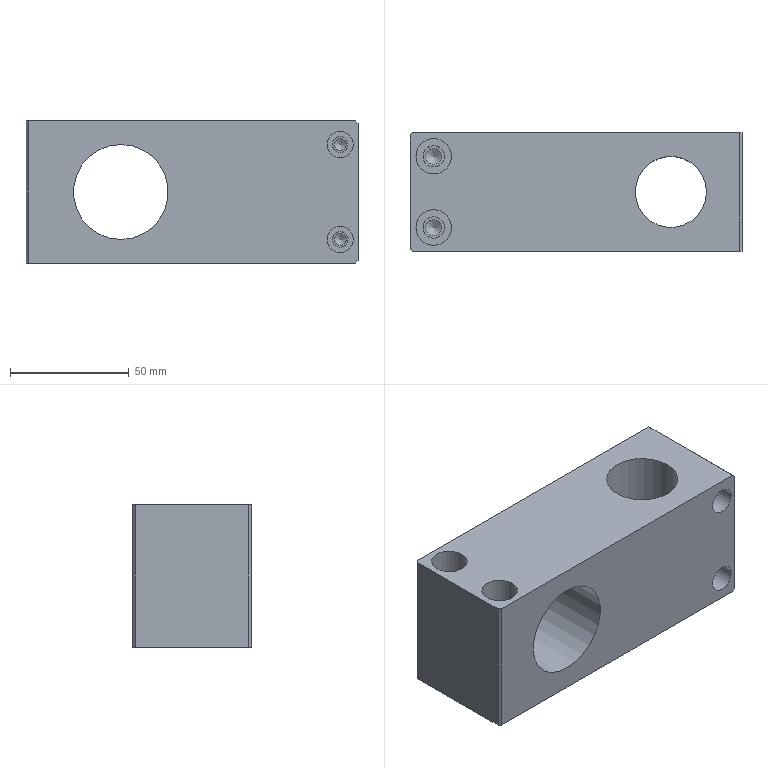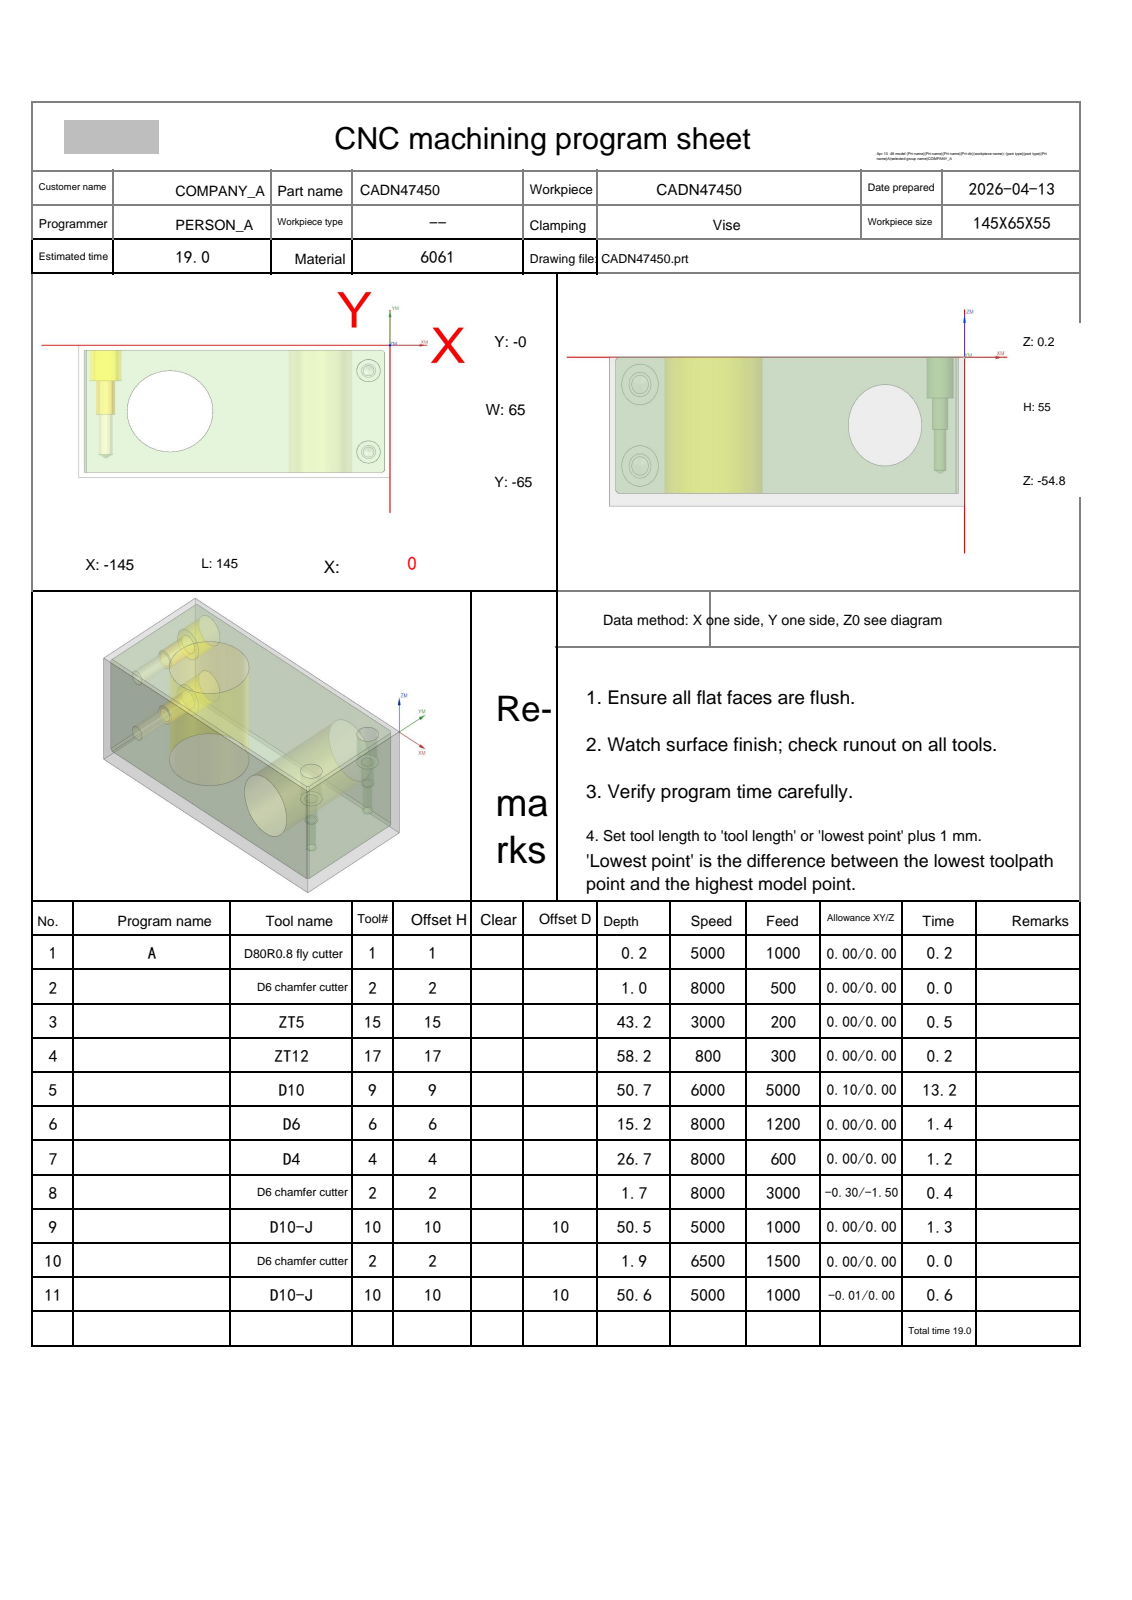NC program | NX | posted by the shop | part box 140 x 50 x 60 mm
Lines 77 to 885 of 4750:
N5 T09 M06
(D10  D=10. R=0. H=09 ce=0.10 di=0.00)
G00 G90 G54 X-73. Y2.6 M03 S6000
G43 H09 Z20.
M08
Z.5
G01 X-3.5 Z.372 F5000.
G02 X.106 Y1.106 Z.365 I0.0 J-5.1
G01 X1.106 Y.106 Z.362
G02 X2.6 Y-3.5 Z.355 I-3.606 J-3.606
G01 Y-61.5 Z.248
G02 X1.106 Y-65.106 Z.24 I-5.1 J0.0
G01 X.106 Y-66.106 Z.238
G02 X-3.5 Y-67.6 Z.23 I-3.606 J3.606
G01 X-142.5 Z-.026
G02 X-147.6 Y-62.5 Z-.04 I0.0 J5.1
G01 Y-2.5 Z-.151
G02 X-142.5 Y2.6 Z-.166 I5.1 J0.0
G01 X-3.5 Z-.422
G02 X.106 Y1.106 Z-.429 I0.0 J-5.1
G01 X1.106 Y.106 Z-.432
G02 X2.6 Y-3.5 Z-.439 I-3.606 J-3.606
G01 Y-61.5 Z-.546
G02 X1.106 Y-65.106 Z-.553 I-5.1 J0.0
G01 X.106 Y-66.106 Z-.556
G02 X-3.5 Y-67.6 Z-.563 I-3.606 J3.606
G01 X-142.5 Z-.819
G02 X-147.6 Y-62.5 Z-.834 I0.0 J5.1
G01 Y-2.5 Z-.945
G02 X-142.5 Y2.6 Z-.959 I5.1 J0.0
G01 X-3.5 Z-1.216
G02 X.106 Y1.106 Z-1.223 I0.0 J-5.1
G01 X1.106 Y.106 Z-1.226
G02 X2.6 Y-3.5 Z-1.233 I-3.606 J-3.606
G01 Y-61.5 Z-1.34
G02 X1.106 Y-65.106 Z-1.347 I-5.1 J0.0
G01 X.106 Y-66.106 Z-1.35
G02 X-3.5 Y-67.6 Z-1.357 I-3.606 J3.606
G01 X-142.5 Z-1.613
G02 X-147.6 Y-62.5 Z-1.628 I0.0 J5.1
G01 Y-2.5 Z-1.738
G02 X-142.5 Y2.6 Z-1.753 I5.1 J0.0
G01 X-3.5 Z-2.009
G02 X.106 Y1.106 Z-2.017 I0.0 J-5.1
G01 X1.106 Y.106 Z-2.019
G02 X2.6 Y-3.5 Z-2.027 I-3.606 J-3.606
G01 Y-61.5 Z-2.133
G02 X1.106 Y-65.106 Z-2.141 I-5.1 J0.0
G01 X.106 Y-66.106 Z-2.143
G02 X-3.5 Y-67.6 Z-2.151 I-3.606 J3.606
G01 X-142.5 Z-2.407
G02 X-147.6 Y-62.5 Z-2.422 I0.0 J5.1
G01 Y-2.5 Z-2.532
G02 X-142.5 Y2.6 Z-2.547 I5.1 J0.0
G01 X-3.5 Z-2.803
G02 X.106 Y1.106 Z-2.81 I0.0 J-5.1
G01 X1.106 Y.106 Z-2.813
G02 X2.6 Y-3.5 Z-2.82 I-3.606 J-3.606
G01 Y-61.5 Z-2.927
G02 X1.106 Y-65.106 Z-2.935 I-5.1 J0.0
G01 X.106 Y-66.106 Z-2.937
G02 X-3.5 Y-67.6 Z-2.945 I-3.606 J3.606
G01 X-142.5 Z-3.201
G02 X-147.6 Y-62.5 Z-3.215 I0.0 J5.1
G01 Y-2.5 Z-3.326
G02 X-142.5 Y2.6 Z-3.341 I5.1 J0.0
G01 X-3.5 Z-3.597
G02 X.106 Y1.106 Z-3.604 I0.0 J-5.1
G01 X1.106 Y.106 Z-3.607
G02 X2.6 Y-3.5 Z-3.614 I-3.606 J-3.606
G01 Y-61.5 Z-3.721
G02 X1.106 Y-65.106 Z-3.728 I-5.1 J0.0
G01 X.106 Y-66.106 Z-3.731
G02 X-3.5 Y-67.6 Z-3.738 I-3.606 J3.606
G01 X-142.5 Z-3.994
G02 X-147.6 Y-62.5 Z-4.009 I0.0 J5.1
G01 Y-2.5 Z-4.12
G02 X-142.5 Y2.6 Z-4.134 I5.1 J0.0
G01 X-3.5 Z-4.391
G02 X.106 Y1.106 Z-4.398 I0.0 J-5.1
G01 X1.106 Y.106 Z-4.401
G02 X2.6 Y-3.5 Z-4.408 I-3.606 J-3.606
G01 Y-61.5 Z-4.515
G02 X1.106 Y-65.106 Z-4.522 I-5.1 J0.0
G01 X.106 Y-66.106 Z-4.525
G02 X-3.5 Y-67.6 Z-4.532 I-3.606 J3.606
G01 X-142.5 Z-4.788
G02 X-147.6 Y-62.5 Z-4.803 I0.0 J5.1
G01 Y-2.5 Z-4.913
G02 X-142.5 Y2.6 Z-4.928 I5.1 J0.0
G01 X-3.5 Z-5.184
G02 X.106 Y1.106 Z-5.192 I0.0 J-5.1
G01 X1.106 Y.106 Z-5.194
G02 X2.6 Y-3.5 Z-5.202 I-3.606 J-3.606
G01 Y-61.5 Z-5.308
G02 X1.106 Y-65.106 Z-5.316 I-5.1 J0.0
G01 X.106 Y-66.106 Z-5.318
G02 X-3.5 Y-67.6 Z-5.326 I-3.606 J3.606
G01 X-142.5 Z-5.582
G02 X-147.6 Y-62.5 Z-5.597 I0.0 J5.1
G01 Y-2.5 Z-5.707
G02 X-142.5 Y2.6 Z-5.722 I5.1 J0.0
G01 X-3.5 Z-5.978
G02 X.106 Y1.106 Z-5.985 I0.0 J-5.1
G01 X1.106 Y.106 Z-5.988
G02 X2.6 Y-3.5 Z-5.995 I-3.606 J-3.606
G01 Y-61.5 Z-6.102
G02 X1.106 Y-65.106 Z-6.11 I-5.1 J0.0
G01 X.106 Y-66.106 Z-6.112
G02 X-3.5 Y-67.6 Z-6.12 I-3.606 J3.606
G01 X-142.5 Z-6.376
G02 X-147.6 Y-62.5 Z-6.39 I0.0 J5.1
G01 Y-2.5 Z-6.501
G02 X-142.5 Y2.6 Z-6.516 I5.1 J0.0
G01 X-3.5 Z-6.772
G02 X.106 Y1.106 Z-6.779 I0.0 J-5.1
G01 X1.106 Y.106 Z-6.782
G02 X2.6 Y-3.5 Z-6.789 I-3.606 J-3.606
G01 Y-61.5 Z-6.896
G02 X1.106 Y-65.106 Z-6.903 I-5.1 J0.0
G01 X.106 Y-66.106 Z-6.906
G02 X-3.5 Y-67.6 Z-6.913 I-3.606 J3.606
G01 X-142.5 Z-7.169
G02 X-147.6 Y-62.5 Z-7.184 I0.0 J5.1
G01 Y-2.5 Z-7.295
G02 X-142.5 Y2.6 Z-7.309 I5.1 J0.0
G01 X-3.5 Z-7.566
G02 X.106 Y1.106 Z-7.573 I0.0 J-5.1
G01 X1.106 Y.106 Z-7.576
G02 X2.6 Y-3.5 Z-7.583 I-3.606 J-3.606
G01 Y-61.5 Z-7.69
G02 X1.106 Y-65.106 Z-7.697 I-5.1 J0.0
G01 X.106 Y-66.106 Z-7.7
G02 X-3.5 Y-67.6 Z-7.707 I-3.606 J3.606
G01 X-142.5 Z-7.963
G02 X-147.6 Y-62.5 Z-7.978 I0.0 J5.1
G01 Y-2.5 Z-8.088
G02 X-142.5 Y2.6 Z-8.103 I5.1 J0.0
G01 X-3.5 Z-8.359
G02 X.106 Y1.106 Z-8.367 I0.0 J-5.1
G01 X1.106 Y.106 Z-8.369
G02 X2.6 Y-3.5 Z-8.377 I-3.606 J-3.606
G01 Y-61.5 Z-8.483
G02 X1.106 Y-65.106 Z-8.491 I-5.1 J0.0
G01 X.106 Y-66.106 Z-8.493
G02 X-3.5 Y-67.6 Z-8.501 I-3.606 J3.606
G01 X-142.5 Z-8.757
G02 X-147.6 Y-62.5 Z-8.772 I0.0 J5.1
G01 Y-2.5 Z-8.882
G02 X-142.5 Y2.6 Z-8.897 I5.1 J0.0
G01 X-3.5 Z-9.153
G02 X.106 Y1.106 Z-9.16 I0.0 J-5.1
G01 X1.106 Y.106 Z-9.163
G02 X2.6 Y-3.5 Z-9.17 I-3.606 J-3.606
G01 Y-61.5 Z-9.277
G02 X1.106 Y-65.106 Z-9.285 I-5.1 J0.0
G01 X.106 Y-66.106 Z-9.287
G02 X-3.5 Y-67.6 Z-9.295 I-3.606 J3.606
G01 X-142.5 Z-9.551
G02 X-147.6 Y-62.5 Z-9.565 I0.0 J5.1
G01 Y-2.5 Z-9.676
G02 X-142.5 Y2.6 Z-9.691 I5.1 J0.0
G01 X-3.5 Z-9.947
G02 X.106 Y1.106 Z-9.954 I0.0 J-5.1
G01 X1.106 Y.106 Z-9.957
G02 X2.6 Y-3.5 Z-9.964 I-3.606 J-3.606
G01 Y-61.5 Z-10.071
G02 X1.106 Y-65.106 Z-10.078 I-5.1 J0.0
G01 X.106 Y-66.106 Z-10.081
G02 X-3.5 Y-67.6 Z-10.088 I-3.606 J3.606
G01 X-142.5 Z-10.344
G02 X-147.6 Y-62.5 Z-10.359 I0.0 J5.1
G01 Y-2.5 Z-10.47
G02 X-142.5 Y2.6 Z-10.484 I5.1 J0.0
G01 X-3.5 Z-10.741
G02 X.106 Y1.106 Z-10.748 I0.0 J-5.1
G01 X1.106 Y.106 Z-10.751
G02 X2.6 Y-3.5 Z-10.758 I-3.606 J-3.606
G01 Y-61.5 Z-10.865
G02 X1.106 Y-65.106 Z-10.872 I-5.1 J0.0
G01 X.106 Y-66.106 Z-10.875
G02 X-3.5 Y-67.6 Z-10.882 I-3.606 J3.606
G01 X-142.5 Z-11.138
G02 X-147.6 Y-62.5 Z-11.153 I0.0 J5.1
G01 Y-2.5 Z-11.263
G02 X-142.5 Y2.6 Z-11.278 I5.1 J0.0
G01 X-3.5 Z-11.534
G02 X.106 Y1.106 Z-11.542 I0.0 J-5.1
G01 X1.106 Y.106 Z-11.544
G02 X2.6 Y-3.5 Z-11.552 I-3.606 J-3.606
G01 Y-61.5 Z-11.658
G02 X1.106 Y-65.106 Z-11.666 I-5.1 J0.0
G01 X.106 Y-66.106 Z-11.668
G02 X-3.5 Y-67.6 Z-11.676 I-3.606 J3.606
G01 X-142.5 Z-11.932
G02 X-147.6 Y-62.5 Z-11.947 I0.0 J5.1
G01 Y-2.5 Z-12.057
G02 X-142.5 Y2.6 Z-12.072 I5.1 J0.0
G01 X-3.5 Z-12.328
G02 X.106 Y1.106 Z-12.335 I0.0 J-5.1
G01 X1.106 Y.106 Z-12.338
G02 X2.6 Y-3.5 Z-12.345 I-3.606 J-3.606
G01 Y-61.5 Z-12.452
G02 X1.106 Y-65.106 Z-12.46 I-5.1 J0.0
G01 X.106 Y-66.106 Z-12.462
G02 X-3.5 Y-67.6 Z-12.47 I-3.606 J3.606
G01 X-142.5 Z-12.726
G02 X-147.6 Y-62.5 Z-12.74 I0.0 J5.1
G01 Y-2.5 Z-12.851
G02 X-142.5 Y2.6 Z-12.866 I5.1 J0.0
G01 X-3.5 Z-13.122
G02 X.106 Y1.106 Z-13.129 I0.0 J-5.1
G01 X1.106 Y.106 Z-13.132
G02 X2.6 Y-3.5 Z-13.139 I-3.606 J-3.606
G01 Y-61.5 Z-13.246
G02 X1.106 Y-65.106 Z-13.253 I-5.1 J0.0
G01 X.106 Y-66.106 Z-13.256
G02 X-3.5 Y-67.6 Z-13.263 I-3.606 J3.606
G01 X-142.5 Z-13.519
G02 X-147.6 Y-62.5 Z-13.534 I0.0 J5.1
G01 Y-2.5 Z-13.645
G02 X-142.5 Y2.6 Z-13.659 I5.1 J0.0
G01 X-3.5 Z-13.916
G02 X.106 Y1.106 Z-13.923 I0.0 J-5.1
G01 X1.106 Y.106 Z-13.926
G02 X2.6 Y-3.5 Z-13.933 I-3.606 J-3.606
G01 Y-61.5 Z-14.04
G02 X1.106 Y-65.106 Z-14.047 I-5.1 J0.0
G01 X.106 Y-66.106 Z-14.05
G02 X-3.5 Y-67.6 Z-14.057 I-3.606 J3.606
G01 X-142.5 Z-14.313
G02 X-147.6 Y-62.5 Z-14.328 I0.0 J5.1
G01 Y-2.5 Z-14.438
G02 X-142.5 Y2.6 Z-14.453 I5.1 J0.0
G01 X-3.5 Z-14.709
G02 X.106 Y1.106 Z-14.717 I0.0 J-5.1
G01 X1.106 Y.106 Z-14.719
G02 X2.6 Y-3.5 Z-14.727 I-3.606 J-3.606
G01 Y-61.5 Z-14.833
G02 X1.106 Y-65.106 Z-14.841 I-5.1 J0.0
G01 X.106 Y-66.106 Z-14.843
G02 X-3.5 Y-67.6 Z-14.851 I-3.606 J3.606
G01 X-142.5 Z-15.107
G02 X-147.6 Y-62.5 Z-15.122 I0.0 J5.1
G01 Y-2.5 Z-15.232
G02 X-142.5 Y2.6 Z-15.247 I5.1 J0.0
G01 X-3.5 Z-15.503
G02 X.106 Y1.106 Z-15.51 I0.0 J-5.1
G01 X1.106 Y.106 Z-15.513
G02 X2.6 Y-3.5 Z-15.52 I-3.606 J-3.606
G01 Y-61.5 Z-15.627
G02 X1.106 Y-65.106 Z-15.635 I-5.1 J0.0
G01 X.106 Y-66.106 Z-15.637
G02 X-3.5 Y-67.6 Z-15.645 I-3.606 J3.606
G01 X-142.5 Z-15.901
G02 X-147.6 Y-62.5 Z-15.915 I0.0 J5.1
G01 Y-2.5 Z-16.026
G02 X-142.5 Y2.6 Z-16.041 I5.1 J0.0
G01 X-3.5 Z-16.297
G02 X.106 Y1.106 Z-16.304 I0.0 J-5.1
G01 X1.106 Y.106 Z-16.307
G02 X2.6 Y-3.5 Z-16.314 I-3.606 J-3.606
G01 Y-61.5 Z-16.421
G02 X1.106 Y-65.106 Z-16.428 I-5.1 J0.0
G01 X.106 Y-66.106 Z-16.431
G02 X-3.5 Y-67.6 Z-16.438 I-3.606 J3.606
G01 X-142.5 Z-16.694
G02 X-147.6 Y-62.5 Z-16.709 I0.0 J5.1
G01 Y-2.5 Z-16.82
G02 X-142.5 Y2.6 Z-16.834 I5.1 J0.0
G01 X-3.5 Z-17.091
G02 X.106 Y1.106 Z-17.098 I0.0 J-5.1
G01 X1.106 Y.106 Z-17.101
G02 X2.6 Y-3.5 Z-17.108 I-3.606 J-3.606
G01 Y-61.5 Z-17.215
G02 X1.106 Y-65.106 Z-17.222 I-5.1 J0.0
G01 X.106 Y-66.106 Z-17.225
G02 X-3.5 Y-67.6 Z-17.232 I-3.606 J3.606
G01 X-142.5 Z-17.488
G02 X-147.6 Y-62.5 Z-17.503 I0.0 J5.1
G01 Y-2.5 Z-17.613
G02 X-142.5 Y2.6 Z-17.628 I5.1 J0.0
G01 X-3.5 Z-17.884
G02 X.106 Y1.106 Z-17.892 I0.0 J-5.1
G01 X1.106 Y.106 Z-17.894
G02 X2.6 Y-3.5 Z-17.902 I-3.606 J-3.606
G01 Y-61.5 Z-18.008
G02 X1.106 Y-65.106 Z-18.016 I-5.1 J0.0
G01 X.106 Y-66.106 Z-18.018
G02 X-3.5 Y-67.6 Z-18.026 I-3.606 J3.606
G01 X-142.5 Z-18.282
G02 X-147.6 Y-62.5 Z-18.297 I0.0 J5.1
G01 Y-2.5 Z-18.407
G02 X-142.5 Y2.6 Z-18.422 I5.1 J0.0
G01 X-3.5 Z-18.678
G02 X.106 Y1.106 Z-18.685 I0.0 J-5.1
G01 X1.106 Y.106 Z-18.688
G02 X2.6 Y-3.5 Z-18.695 I-3.606 J-3.606
G01 Y-61.5 Z-18.802
G02 X1.106 Y-65.106 Z-18.81 I-5.1 J0.0
G01 X.106 Y-66.106 Z-18.812
G02 X-3.5 Y-67.6 Z-18.82 I-3.606 J3.606
G01 X-142.5 Z-19.076
G02 X-147.6 Y-62.5 Z-19.09 I0.0 J5.1
G01 Y-2.5 Z-19.201
G02 X-142.5 Y2.6 Z-19.216 I5.1 J0.0
G01 X-3.5 Z-19.472
G02 X.106 Y1.106 Z-19.479 I0.0 J-5.1
G01 X1.106 Y.106 Z-19.482
G02 X2.6 Y-3.5 Z-19.489 I-3.606 J-3.606
G01 Y-61.5 Z-19.596
G02 X1.106 Y-65.106 Z-19.603 I-5.1 J0.0
G01 X.106 Y-66.106 Z-19.606
G02 X-3.5 Y-67.6 Z-19.613 I-3.606 J3.606
G01 X-142.5 Z-19.869
G02 X-147.6 Y-62.5 Z-19.884 I0.0 J5.1
G01 Y-2.5 Z-19.995
G02 X-142.5 Y2.6 Z-20.009 I5.1 J0.0
G01 X-3.5 Z-20.266
G02 X.106 Y1.106 Z-20.273 I0.0 J-5.1
G01 X1.106 Y.106 Z-20.276
G02 X2.6 Y-3.5 Z-20.283 I-3.606 J-3.606
G01 Y-61.5 Z-20.39
G02 X1.106 Y-65.106 Z-20.397 I-5.1 J0.0
G01 X.106 Y-66.106 Z-20.4
G02 X-3.5 Y-67.6 Z-20.407 I-3.606 J3.606
G01 X-142.5 Z-20.663
G02 X-147.6 Y-62.5 Z-20.678 I0.0 J5.1
G01 Y-2.5 Z-20.788
G02 X-142.5 Y2.6 Z-20.803 I5.1 J0.0
G01 X-3.5 Z-21.059
G02 X.106 Y1.106 Z-21.067 I0.0 J-5.1
G01 X1.106 Y.106 Z-21.069
G02 X2.6 Y-3.5 Z-21.077 I-3.606 J-3.606
G01 Y-61.5 Z-21.183
G02 X1.106 Y-65.106 Z-21.191 I-5.1 J0.0
G01 X.106 Y-66.106 Z-21.193
G02 X-3.5 Y-67.6 Z-21.201 I-3.606 J3.606
G01 X-142.5 Z-21.457
G02 X-147.6 Y-62.5 Z-21.472 I0.0 J5.1
G01 Y-2.5 Z-21.582
G02 X-142.5 Y2.6 Z-21.597 I5.1 J0.0
G01 X-3.5 Z-21.853
G02 X.106 Y1.106 Z-21.86 I0.0 J-5.1
G01 X1.106 Y.106 Z-21.863
G02 X2.6 Y-3.5 Z-21.87 I-3.606 J-3.606
G01 Y-61.5 Z-21.977
G02 X1.106 Y-65.106 Z-21.985 I-5.1 J0.0
G01 X.106 Y-66.106 Z-21.987
G02 X-3.5 Y-67.6 Z-21.995 I-3.606 J3.606
G01 X-142.5 Z-22.251
G02 X-147.6 Y-62.5 Z-22.265 I0.0 J5.1
G01 Y-2.5 Z-22.376
G02 X-142.5 Y2.6 Z-22.391 I5.1 J0.0
G01 X-3.5 Z-22.647
G02 X.106 Y1.106 Z-22.654 I0.0 J-5.1
G01 X1.106 Y.106 Z-22.657
G02 X2.6 Y-3.5 Z-22.664 I-3.606 J-3.606
G01 Y-61.5 Z-22.771
G02 X1.106 Y-65.106 Z-22.778 I-5.1 J0.0
G01 X.106 Y-66.106 Z-22.781
G02 X-3.5 Y-67.6 Z-22.788 I-3.606 J3.606
G01 X-142.5 Z-23.044
G02 X-147.6 Y-62.5 Z-23.059 I0.0 J5.1
G01 Y-2.5 Z-23.17
G02 X-142.5 Y2.6 Z-23.184 I5.1 J0.0
G01 X-3.5 Z-23.441
G02 X.106 Y1.106 Z-23.448 I0.0 J-5.1
G01 X1.106 Y.106 Z-23.451
G02 X2.6 Y-3.5 Z-23.458 I-3.606 J-3.606
G01 Y-61.5 Z-23.565
G02 X1.106 Y-65.106 Z-23.572 I-5.1 J0.0
G01 X.106 Y-66.106 Z-23.575
G02 X-3.5 Y-67.6 Z-23.582 I-3.606 J3.606
G01 X-142.5 Z-23.838
G02 X-147.6 Y-62.5 Z-23.853 I0.0 J5.1
G01 Y-2.5 Z-23.963
G02 X-142.5 Y2.6 Z-23.978 I5.1 J0.0
G01 X-3.5 Z-24.234
G02 X.106 Y1.106 Z-24.242 I0.0 J-5.1
G01 X1.106 Y.106 Z-24.244
G02 X2.6 Y-3.5 Z-24.252 I-3.606 J-3.606
G01 Y-61.5 Z-24.358
G02 X1.106 Y-65.106 Z-24.366 I-5.1 J0.0
G01 X.106 Y-66.106 Z-24.368
G02 X-3.5 Y-67.6 Z-24.376 I-3.606 J3.606
G01 X-142.5 Z-24.632
G02 X-147.6 Y-62.5 Z-24.647 I0.0 J5.1
G01 Y-2.5 Z-24.757
G02 X-142.5 Y2.6 Z-24.772 I5.1 J0.0
G01 X-3.5 Z-25.028
G02 X.106 Y1.106 Z-25.035 I0.0 J-5.1
G01 X1.106 Y.106 Z-25.038
G02 X2.6 Y-3.5 Z-25.045 I-3.606 J-3.606
G01 Y-61.5 Z-25.152
G02 X1.106 Y-65.106 Z-25.16 I-5.1 J0.0
G01 X.106 Y-66.106 Z-25.162
G02 X-3.5 Y-67.6 Z-25.17 I-3.606 J3.606
G01 X-142.5 Z-25.426
G02 X-147.6 Y-62.5 Z-25.44 I0.0 J5.1
G01 Y-2.5 Z-25.551
G02 X-142.5 Y2.6 Z-25.566 I5.1 J0.0
G01 X-3.5 Z-25.822
G02 X.106 Y1.106 Z-25.829 I0.0 J-5.1
G01 X1.106 Y.106 Z-25.832
G02 X2.6 Y-3.5 Z-25.839 I-3.606 J-3.606
G01 Y-61.5 Z-25.946
G02 X1.106 Y-65.106 Z-25.953 I-5.1 J0.0
G01 X.106 Y-66.106 Z-25.956
G02 X-3.5 Y-67.6 Z-25.963 I-3.606 J3.606
G01 X-142.5 Z-26.219
G02 X-147.6 Y-62.5 Z-26.234 I0.0 J5.1
G01 Y-2.5 Z-26.345
G02 X-142.5 Y2.6 Z-26.359 I5.1 J0.0
G01 X-3.5 Z-26.616
G02 X.106 Y1.106 Z-26.623 I0.0 J-5.1
G01 X1.106 Y.106 Z-26.626
G02 X2.6 Y-3.5 Z-26.633 I-3.606 J-3.606
G01 Y-61.5 Z-26.74
G02 X1.106 Y-65.106 Z-26.747 I-5.1 J0.0
G01 X.106 Y-66.106 Z-26.75
G02 X-3.5 Y-67.6 Z-26.757 I-3.606 J3.606
G01 X-142.5 Z-27.013
G02 X-147.6 Y-62.5 Z-27.028 I0.0 J5.1
G01 Y-2.5 Z-27.138
G02 X-142.5 Y2.6 Z-27.153 I5.1 J0.0
G01 X-3.5 Z-27.409
G02 X.106 Y1.106 Z-27.417 I0.0 J-5.1
G01 X1.106 Y.106 Z-27.419
G02 X2.6 Y-3.5 Z-27.427 I-3.606 J-3.606
G01 Y-61.5 Z-27.533
G02 X1.106 Y-65.106 Z-27.541 I-5.1 J0.0
G01 X.106 Y-66.106 Z-27.543
G02 X-3.5 Y-67.6 Z-27.551 I-3.606 J3.606
G01 X-142.5 Z-27.807
G02 X-147.6 Y-62.5 Z-27.822 I0.0 J5.1
G01 Y-2.5 Z-27.932
G02 X-142.5 Y2.6 Z-27.947 I5.1 J0.0
G01 X-3.5 Z-28.203
G02 X.106 Y1.106 Z-28.21 I0.0 J-5.1
G01 X1.106 Y.106 Z-28.213
G02 X2.6 Y-3.5 Z-28.22 I-3.606 J-3.606
G01 Y-61.5 Z-28.327
G02 X1.106 Y-65.106 Z-28.335 I-5.1 J0.0
G01 X.106 Y-66.106 Z-28.337
G02 X-3.5 Y-67.6 Z-28.345 I-3.606 J3.606
G01 X-142.5 Z-28.601
G02 X-147.6 Y-62.5 Z-28.615 I0.0 J5.1
G01 Y-2.5 Z-28.726
G02 X-142.5 Y2.6 Z-28.741 I5.1 J0.0
G01 X-3.5 Z-28.997
G02 X.106 Y1.106 Z-29.004 I0.0 J-5.1
G01 X1.106 Y.106 Z-29.007
G02 X2.6 Y-3.5 Z-29.014 I-3.606 J-3.606
G01 Y-61.5 Z-29.121
G02 X1.106 Y-65.106 Z-29.128 I-5.1 J0.0
G01 X.106 Y-66.106 Z-29.131
G02 X-3.5 Y-67.6 Z-29.138 I-3.606 J3.606
G01 X-142.5 Z-29.394
G02 X-147.6 Y-62.5 Z-29.409 I0.0 J5.1
G01 Y-2.5 Z-29.52
G02 X-142.5 Y2.6 Z-29.534 I5.1 J0.0
G01 X-3.5 Z-29.791
G02 X.106 Y1.106 Z-29.798 I0.0 J-5.1
G01 X1.106 Y.106 Z-29.801
G02 X2.6 Y-3.5 Z-29.808 I-3.606 J-3.606
G01 Y-61.5 Z-29.915
G02 X1.106 Y-65.106 Z-29.922 I-5.1 J0.0
G01 X.106 Y-66.106 Z-29.925
G02 X-3.5 Y-67.6 Z-29.932 I-3.606 J3.606
G01 X-142.5 Z-30.188
G02 X-147.6 Y-62.5 Z-30.203 I0.0 J5.1
G01 Y-2.5 Z-30.313
G02 X-142.5 Y2.6 Z-30.328 I5.1 J0.0
G01 X-3.5 Z-30.584
G02 X.106 Y1.106 Z-30.592 I0.0 J-5.1
G01 X1.106 Y.106 Z-30.594
G02 X2.6 Y-3.5 Z-30.602 I-3.606 J-3.606
G01 Y-61.5 Z-30.708
G02 X1.106 Y-65.106 Z-30.716 I-5.1 J0.0
G01 X.106 Y-66.106 Z-30.718
G02 X-3.5 Y-67.6 Z-30.726 I-3.606 J3.606
G01 X-142.5 Z-30.982
G02 X-147.6 Y-62.5 Z-30.997 I0.0 J5.1
G01 Y-2.5 Z-31.107
G02 X-142.5 Y2.6 Z-31.122 I5.1 J0.0
G01 X-3.5 Z-31.378
G02 X.106 Y1.106 Z-31.385 I0.0 J-5.1
G01 X1.106 Y.106 Z-31.388
G02 X2.6 Y-3.5 Z-31.395 I-3.606 J-3.606
G01 Y-61.5 Z-31.502
G02 X1.106 Y-65.106 Z-31.51 I-5.1 J0.0
G01 X.106 Y-66.106 Z-31.512
G02 X-3.5 Y-67.6 Z-31.52 I-3.606 J3.606
G01 X-142.5 Z-31.776
G02 X-147.6 Y-62.5 Z-31.79 I0.0 J5.1
G01 Y-2.5 Z-31.901
G02 X-142.5 Y2.6 Z-31.916 I5.1 J0.0
G01 X-3.5 Z-32.172
G02 X.106 Y1.106 Z-32.179 I0.0 J-5.1
G01 X1.106 Y.106 Z-32.182
G02 X2.6 Y-3.5 Z-32.189 I-3.606 J-3.606
G01 Y-61.5 Z-32.296
G02 X1.106 Y-65.106 Z-32.303 I-5.1 J0.0
G01 X.106 Y-66.106 Z-32.306
G02 X-3.5 Y-67.6 Z-32.313 I-3.606 J3.606
G01 X-142.5 Z-32.569
G02 X-147.6 Y-62.5 Z-32.584 I0.0 J5.1
G01 Y-2.5 Z-32.695
G02 X-142.5 Y2.6 Z-32.709 I5.1 J0.0
G01 X-3.5 Z-32.966
G02 X.106 Y1.106 Z-32.973 I0.0 J-5.1
G01 X1.106 Y.106 Z-32.976
G02 X2.6 Y-3.5 Z-32.983 I-3.606 J-3.606
G01 Y-61.5 Z-33.09
G02 X1.106 Y-65.106 Z-33.097 I-5.1 J0.0
G01 X.106 Y-66.106 Z-33.1
G02 X-3.5 Y-67.6 Z-33.107 I-3.606 J3.606
G01 X-142.5 Z-33.363
G02 X-147.6 Y-62.5 Z-33.378 I0.0 J5.1
G01 Y-2.5 Z-33.488
G02 X-142.5 Y2.6 Z-33.503 I5.1 J0.0
G01 X-3.5 Z-33.759
G02 X.106 Y1.106 Z-33.767 I0.0 J-5.1
G01 X1.106 Y.106 Z-33.769
G02 X2.6 Y-3.5 Z-33.777 I-3.606 J-3.606
G01 Y-61.5 Z-33.883
G02 X1.106 Y-65.106 Z-33.891 I-5.1 J0.0
G01 X.106 Y-66.106 Z-33.893
G02 X-3.5 Y-67.6 Z-33.901 I-3.606 J3.606
G01 X-142.5 Z-34.157
G02 X-147.6 Y-62.5 Z-34.172 I0.0 J5.1
G01 Y-2.5 Z-34.282
G02 X-142.5 Y2.6 Z-34.297 I5.1 J0.0
G01 X-3.5 Z-34.553
G02 X.106 Y1.106 Z-34.56 I0.0 J-5.1
G01 X1.106 Y.106 Z-34.563
G02 X2.6 Y-3.5 Z-34.57 I-3.606 J-3.606
G01 Y-61.5 Z-34.677
G02 X1.106 Y-65.106 Z-34.685 I-5.1 J0.0
G01 X.106 Y-66.106 Z-34.687
G02 X-3.5 Y-67.6 Z-34.695 I-3.606 J3.606
G01 X-142.5 Z-34.951
G02 X-147.6 Y-62.5 Z-34.965 I0.0 J5.1
G01 Y-2.5 Z-35.076
G02 X-142.5 Y2.6 Z-35.091 I5.1 J0.0
G01 X-3.5 Z-35.347
G02 X.106 Y1.106 Z-35.354 I0.0 J-5.1
G01 X1.106 Y.106 Z-35.357
G02 X2.6 Y-3.5 Z-35.364 I-3.606 J-3.606
G01 Y-61.5 Z-35.471
G02 X1.106 Y-65.106 Z-35.478 I-5.1 J0.0
G01 X.106 Y-66.106 Z-35.481
G02 X-3.5 Y-67.6 Z-35.488 I-3.606 J3.606
G01 X-142.5 Z-35.744
G02 X-147.6 Y-62.5 Z-35.759 I0.0 J5.1
G01 Y-2.5 Z-35.87
G02 X-142.5 Y2.6 Z-35.884 I5.1 J0.0
G01 X-3.5 Z-36.141
G02 X.106 Y1.106 Z-36.148 I0.0 J-5.1
G01 X1.106 Y.106 Z-36.151
G02 X2.6 Y-3.5 Z-36.158 I-3.606 J-3.606
G01 Y-61.5 Z-36.265
G02 X1.106 Y-65.106 Z-36.272 I-5.1 J0.0
G01 X.106 Y-66.106 Z-36.275
G02 X-3.5 Y-67.6 Z-36.282 I-3.606 J3.606
G01 X-142.5 Z-36.538
G02 X-147.6 Y-62.5 Z-36.553 I0.0 J5.1
G01 Y-2.5 Z-36.663
G02 X-142.5 Y2.6 Z-36.678 I5.1 J0.0
G01 X-3.5 Z-36.934
G02 X.106 Y1.106 Z-36.942 I0.0 J-5.1
G01 X1.106 Y.106 Z-36.944
G02 X2.6 Y-3.5 Z-36.952 I-3.606 J-3.606
G01 Y-61.5 Z-37.058
G02 X1.106 Y-65.106 Z-37.066 I-5.1 J0.0
G01 X.106 Y-66.106 Z-37.068
G02 X-3.5 Y-67.6 Z-37.076 I-3.606 J3.606
G01 X-142.5 Z-37.332
G02 X-147.6 Y-62.5 Z-37.347 I0.0 J5.1
G01 Y-2.5 Z-37.457
G02 X-142.5 Y2.6 Z-37.472 I5.1 J0.0
G01 X-3.5 Z-37.728
G02 X.106 Y1.106 Z-37.735 I0.0 J-5.1
G01 X1.106 Y.106 Z-37.738
G02 X2.6 Y-3.5 Z-37.745 I-3.606 J-3.606
G01 Y-61.5 Z-37.852
G02 X1.106 Y-65.106 Z-37.86 I-5.1 J0.0
G01 X.106 Y-66.106 Z-37.862
G02 X-3.5 Y-67.6 Z-37.87 I-3.606 J3.606
G01 X-142.5 Z-38.126
G02 X-147.6 Y-62.5 Z-38.14 I0.0 J5.1
G01 Y-2.5 Z-38.251
G02 X-142.5 Y2.6 Z-38.266 I5.1 J0.0
G01 X-3.5 Z-38.522
G02 X.106 Y1.106 Z-38.529 I0.0 J-5.1
G01 X1.106 Y.106 Z-38.532
G02 X2.6 Y-3.5 Z-38.539 I-3.606 J-3.606
G01 Y-61.5 Z-38.646
G02 X1.106 Y-65.106 Z-38.653 I-5.1 J0.0
G01 X.106 Y-66.106 Z-38.656
G02 X-3.5 Y-67.6 Z-38.663 I-3.606 J3.606
G01 X-142.5 Z-38.919
G02 X-147.6 Y-62.5 Z-38.934 I0.0 J5.1
G01 Y-2.5 Z-39.045
G02 X-142.5 Y2.6 Z-39.059 I5.1 J0.0
G01 X-3.5 Z-39.316
G02 X.106 Y1.106 Z-39.323 I0.0 J-5.1
G01 X1.106 Y.106 Z-39.326
G02 X2.6 Y-3.5 Z-39.333 I-3.606 J-3.606
G01 Y-61.5 Z-39.44
G02 X1.106 Y-65.106 Z-39.447 I-5.1 J0.0
G01 X.106 Y-66.106 Z-39.45
G02 X-3.5 Y-67.6 Z-39.457 I-3.606 J3.606
G01 X-142.5 Z-39.713
G02 X-147.6 Y-62.5 Z-39.728 I0.0 J5.1
G01 Y-2.5 Z-39.838
G02 X-142.5 Y2.6 Z-39.853 I5.1 J0.0
G01 X-3.5 Z-40.109
G02 X.106 Y1.106 Z-40.117 I0.0 J-5.1
G01 X1.106 Y.106 Z-40.119
G02 X2.6 Y-3.5 Z-40.127 I-3.606 J-3.606
G01 Y-61.5 Z-40.233
G02 X1.106 Y-65.106 Z-40.241 I-5.1 J0.0
G01 X.106 Y-66.106 Z-40.243
G02 X-3.5 Y-67.6 Z-40.251 I-3.606 J3.606
G01 X-142.5 Z-40.507
G02 X-147.6 Y-62.5 Z-40.522 I0.0 J5.1
G01 Y-2.5 Z-40.632
G02 X-142.5 Y2.6 Z-40.647 I5.1 J0.0
G01 X-3.5 Z-40.903
G02 X.106 Y1.106 Z-40.91 I0.0 J-5.1
G01 X1.106 Y.106 Z-40.913
G02 X2.6 Y-3.5 Z-40.92 I-3.606 J-3.606
G01 Y-61.5 Z-41.027
G02 X1.106 Y-65.106 Z-41.035 I-5.1 J0.0
G01 X.106 Y-66.106 Z-41.037
G02 X-3.5 Y-67.6 Z-41.045 I-3.606 J3.606
G01 X-142.5 Z-41.301
G02 X-147.6 Y-62.5 Z-41.315 I0.0 J5.1
G01 Y-2.5 Z-41.426
G02 X-142.5 Y2.6 Z-41.441 I5.1 J0.0
G01 X-3.5 Z-41.697
G02 X.106 Y1.106 Z-41.704 I0.0 J-5.1
G01 X1.106 Y.106 Z-41.707
G02 X2.6 Y-3.5 Z-41.714 I-3.606 J-3.606
G01 Y-61.5 Z-41.821
G02 X1.106 Y-65.106 Z-41.828 I-5.1 J0.0
G01 X.106 Y-66.106 Z-41.831
G02 X-3.5 Y-67.6 Z-41.838 I-3.606 J3.606
G01 X-142.5 Z-42.094
G02 X-147.6 Y-62.5 Z-42.109 I0.0 J5.1
G01 Y-2.5 Z-42.22
G02 X-142.5 Y2.6 Z-42.234 I5.1 J0.0
G01 X-3.5 Z-42.491
G02 X.106 Y1.106 Z-42.498 I0.0 J-5.1
G01 X1.106 Y.106 Z-42.501
G02 X2.6 Y-3.5 Z-42.508 I-3.606 J-3.606
G01 Y-61.5 Z-42.615
G02 X1.106 Y-65.106 Z-42.622 I-5.1 J0.0
G01 X.106 Y-66.106 Z-42.625
G02 X-3.5 Y-67.6 Z-42.632 I-3.606 J3.606
G01 X-142.5 Z-42.888
G02 X-147.6 Y-62.5 Z-42.903 I0.0 J5.1
G01 Y-2.5 Z-43.013
G02 X-142.5 Y2.6 Z-43.028 I5.1 J0.0
G01 X-3.5 Z-43.284
G02 X.106 Y1.106 Z-43.292 I0.0 J-5.1
G01 X1.106 Y.106 Z-43.294
G02 X2.6 Y-3.5 Z-43.302 I-3.606 J-3.606
G01 Y-61.5 Z-43.408
G02 X1.106 Y-65.106 Z-43.416 I-5.1 J0.0
G01 X.106 Y-66.106 Z-43.418
G02 X-3.5 Y-67.6 Z-43.426 I-3.606 J3.606
G01 X-142.5 Z-43.682
G02 X-147.6 Y-62.5 Z-43.697 I0.0 J5.1
G01 Y-2.5 Z-43.807
G02 X-142.5 Y2.6 Z-43.822 I5.1 J0.0
G01 X-3.5 Z-44.078
G02 X.106 Y1.106 Z-44.085 I0.0 J-5.1
G01 X1.106 Y.106 Z-44.088
G02 X2.6 Y-3.5 Z-44.095 I-3.606 J-3.606
G01 Y-61.5 Z-44.202
G02 X1.106 Y-65.106 Z-44.21 I-5.1 J0.0
G01 X.106 Y-66.106 Z-44.212
G02 X-3.5 Y-67.6 Z-44.22 I-3.606 J3.606
G01 X-142.5 Z-44.476
G02 X-147.6 Y-62.5 Z-44.49 I0.0 J5.1
G01 Y-2.5 Z-44.601
G02 X-142.5 Y2.6 Z-44.616 I5.1 J0.0
G01 X-3.5 Z-44.872
G02 X.106 Y1.106 Z-44.879 I0.0 J-5.1
G01 X1.106 Y.106 Z-44.882
G02 X2.6 Y-3.5 Z-44.889 I-3.606 J-3.606
G01 Y-61.5 Z-44.996
G02 X1.106 Y-65.106 Z-45.003 I-5.1 J0.0
G01 X.106 Y-66.106 Z-45.006
G02 X-3.5 Y-67.6 Z-45.013 I-3.606 J3.606
G01 X-142.5 Z-45.269
G02 X-147.6 Y-62.5 Z-45.284 I0.0 J5.1
G01 Y-2.5 Z-45.395
G02 X-142.5 Y2.6 Z-45.409 I5.1 J0.0
G01 X-3.5 Z-45.666
G02 X.106 Y1.106 Z-45.673 I0.0 J-5.1
G01 X1.106 Y.106 Z-45.676
G02 X2.6 Y-3.5 Z-45.683 I-3.606 J-3.606
G01 Y-61.5 Z-45.79
G02 X1.106 Y-65.106 Z-45.797 I-5.1 J0.0
G01 X.106 Y-66.106 Z-45.8
G02 X-3.5 Y-67.6 Z-45.807 I-3.606 J3.606
G01 X-142.5 Z-46.063
G02 X-147.6 Y-62.5 Z-46.078 I0.0 J5.1
G01 Y-2.5 Z-46.188
G02 X-142.5 Y2.6 Z-46.203 I5.1 J0.0
G01 X-3.5 Z-46.459
G02 X.106 Y1.106 Z-46.467 I0.0 J-5.1
G01 X1.106 Y.106 Z-46.469
G02 X2.6 Y-3.5 Z-46.477 I-3.606 J-3.606
G01 Y-61.5 Z-46.583
G02 X1.106 Y-65.106 Z-46.591 I-5.1 J0.0
G01 X.106 Y-66.106 Z-46.593
G02 X-3.5 Y-67.6 Z-46.601 I-3.606 J3.606
G01 X-142.5 Z-46.857
G02 X-147.6 Y-62.5 Z-46.872 I0.0 J5.1
G01 Y-2.5 Z-46.982
G02 X-142.5 Y2.6 Z-46.997 I5.1 J0.0
G01 X-3.5 Z-47.253
G02 X.106 Y1.106 Z-47.26 I0.0 J-5.1
G01 X1.106 Y.106 Z-47.263
G02 X2.6 Y-3.5 Z-47.27 I-3.606 J-3.606
G01 Y-61.5 Z-47.377
G02 X1.106 Y-65.106 Z-47.385 I-5.1 J0.0
G01 X.106 Y-66.106 Z-47.387
G02 X-3.5 Y-67.6 Z-47.395 I-3.606 J3.606
G01 X-142.5 Z-47.651
G02 X-147.6 Y-62.5 Z-47.665 I0.0 J5.1
G01 Y-2.5 Z-47.776
G02 X-142.5 Y2.6 Z-47.791 I5.1 J0.0
G01 X-3.5 Z-48.047
G02 X.106 Y1.106 Z-48.054 I0.0 J-5.1
G01 X1.106 Y.106 Z-48.057
G02 X2.6 Y-3.5 Z-48.064 I-3.606 J-3.606
G01 Y-61.5 Z-48.171
G02 X1.106 Y-65.106 Z-48.178 I-5.1 J0.0
G01 X.106 Y-66.106 Z-48.181
G02 X-3.5 Y-67.6 Z-48.188 I-3.606 J3.606
G01 X-142.5 Z-48.444
G02 X-147.6 Y-62.5 Z-48.459 I0.0 J5.1
G01 Y-2.5 Z-48.57
G02 X-142.5 Y2.6 Z-48.584 I5.1 J0.0
G01 X-3.5 Z-48.841
G02 X.106 Y1.106 Z-48.848 I0.0 J-5.1
G01 X1.106 Y.106 Z-48.851
G02 X2.6 Y-3.5 Z-48.858 I-3.606 J-3.606
G01 Y-61.5 Z-48.965
G02 X1.106 Y-65.106 Z-48.972 I-5.1 J0.0
G01 X.106 Y-66.106 Z-48.975
G02 X-3.5 Y-67.6 Z-48.982 I-3.606 J3.606
G01 X-142.5 Z-49.238
G02 X-147.6 Y-62.5 Z-49.253 I0.0 J5.1
G01 Y-2.5 Z-49.363
G02 X-142.5 Y2.6 Z-49.378 I5.1 J0.0
G01 X-3.5 Z-49.634
G02 X.106 Y1.106 Z-49.642 I0.0 J-5.1
G01 X1.106 Y.106 Z-49.644
G02 X2.6 Y-3.5 Z-49.652 I-3.606 J-3.606
G01 Y-61.5 Z-49.758
G02 X1.106 Y-65.106 Z-49.766 I-5.1 J0.0
G01 X.106 Y-66.106 Z-49.768
G02 X-3.5 Y-67.6 Z-49.776 I-3.606 J3.606
G01 X-142.5 Z-50.032
G02 X-147.6 Y-62.5 Z-50.047 I0.0 J5.1
G01 Y-2.5 Z-50.157
G02 X-142.5 Y2.6 Z-50.172 I5.1 J0.0
G01 X-73. Z-50.3
X-3.5
G02 X.106 Y1.106 I0.0 J-5.1
G01 X1.106 Y.106
G02 X2.6 Y-3.5 I-3.606 J-3.606
G01 Y-61.5
G02 X1.106 Y-65.106 I-5.1 J0.0
G01 X.106 Y-66.106
G02 X-3.5 Y-67.6 I-3.606 J3.606
G01 X-142.5
G02 X-147.6 Y-62.5 I0.0 J5.1
G01 Y-2.5
G02 X-142.5 Y2.6 I5.1 J0.0
G01 X-73.
X-72.5
Z-49.3
G00 Z20.
G00 G90 X-101.034 Y-37.645 M03 S6000
Z10.2
Z1.5
G02 X-101.034 Y-37.645 Z.018 I-1.466 J-4.255 F3000.
X-99.913 Y-45.582 Z-.5 I-1.466 J-4.255
G01 X-102.5 Y-47.4
G02 X-117.4 Y-32.5 I0.0 J14.9
X-102.5 Y-17.6 I14.9 J0.0
X-87.6 Y-32.5 I0.0 J-14.9
X-102.5 Y-47.4 I-14.9 J0.0
X-107.407 Y-46.569 I0.0 J14.9
X-108.077 Y-45.625 I.329 J.944
G01 X-108.071 Y-45.51
X-107.356 Y-39.322
X-107.35 Y-39.207
G03 X-107.692 Y-38.454 I-1. J0.0
G02 X-110.4 Y-32.5 I5.192 J5.954
X-102.5 Y-24.6 I7.9 J0.0